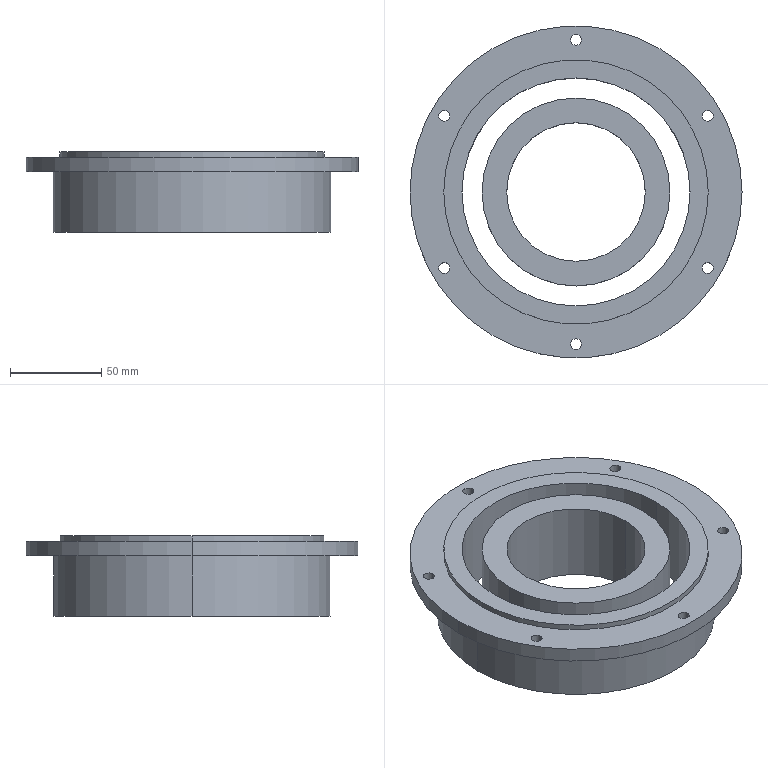Part | STEP file | Encoder | 2 solids | 30 faces | box 182 x 182 x 44 mm | volume 482174 mm3 | cylinder 24 | plane 6 | commonest cylinder face diameters 6 x12 76 x2 103 x2 125 x2 145 x2 152 x2
STEP:
#1=CARTESIAN_POINT('',(-51.5,0.,44.));
#2=VERTEX_POINT('',#1);
#3=CARTESIAN_POINT('',(51.5,0.,44.));
#4=VERTEX_POINT('',#3);
#5=CARTESIAN_POINT('',(0.,0.,44.));
#6=DIRECTION('',(0.,0.,-1.));
#7=DIRECTION('',(-1.,0.,0.));
#8=AXIS2_PLACEMENT_3D('',#5,#6,#7);
#9=CIRCLE('',#8,51.5);
#10=EDGE_CURVE('',#2,#4,#9,.T.);
#11=ORIENTED_EDGE('',*,*,#10,.T.);
#12=CARTESIAN_POINT('',(51.5,0.,0.));
#13=VERTEX_POINT('',#12);
#14=CARTESIAN_POINT('',(51.5,0.,44.));
#15=DIRECTION('',(0.,0.,-1.));
#16=VECTOR('',#15,1000.);
#17=LINE('',#14,#16);
#18=EDGE_CURVE('',#4,#13,#17,.T.);
#19=ORIENTED_EDGE('',*,*,#18,.T.);
#20=CARTESIAN_POINT('',(-51.5,0.,0.));
#21=VERTEX_POINT('',#20);
#22=CARTESIAN_POINT('',(0.,0.,0.));
#23=DIRECTION('',(0.,0.,1.));
#24=DIRECTION('',(-1.,0.,0.));
#25=AXIS2_PLACEMENT_3D('',#22,#23,#24);
#26=CIRCLE('',#25,51.5);
#27=EDGE_CURVE('',#13,#21,#26,.T.);
#28=ORIENTED_EDGE('',*,*,#27,.T.);
#29=CARTESIAN_POINT('',(-51.5,0.,44.));
#30=DIRECTION('',(0.,0.,-1.));
#31=VECTOR('',#30,1000.);
#32=LINE('',#29,#31);
#33=EDGE_CURVE('',#2,#21,#32,.T.);
#34=ORIENTED_EDGE('',*,*,#33,.F.);
#35=EDGE_LOOP('',(#11,#19,#28,#34));
#36=FACE_OUTER_BOUND('',#35,.T.);
#37=CARTESIAN_POINT('',(0.,0.,44.));
#38=DIRECTION('',(0.,0.,-1.));
#39=DIRECTION('',(-1.,0.,0.));
#40=AXIS2_PLACEMENT_3D('',#37,#38,#39);
#41=CYLINDRICAL_SURFACE('',#40,51.5);
#42=ADVANCED_FACE('',(#36),#41,.T.);
#43=CARTESIAN_POINT('',(38.,0.,44.));
#44=VERTEX_POINT('',#43);
#45=CARTESIAN_POINT('',(-38.,0.,44.));
#46=VERTEX_POINT('',#45);
#47=CARTESIAN_POINT('',(0.,0.,44.));
#48=DIRECTION('',(0.,0.,-1.));
#49=DIRECTION('',(-1.,0.,0.));
#50=AXIS2_PLACEMENT_3D('',#47,#48,#49);
#51=CIRCLE('',#50,38.);
#52=EDGE_CURVE('',#44,#46,#51,.T.);
#53=ORIENTED_EDGE('',*,*,#52,.F.);
#54=CARTESIAN_POINT('',(38.,0.,0.));
#55=VERTEX_POINT('',#54);
#56=CARTESIAN_POINT('',(38.,0.,41.));
#57=DIRECTION('',(0.,0.,-1.));
#58=VECTOR('',#57,1000.);
#59=LINE('',#56,#58);
#60=EDGE_CURVE('',#44,#55,#59,.T.);
#61=ORIENTED_EDGE('',*,*,#60,.T.);
#62=CARTESIAN_POINT('',(-38.,0.,0.));
#63=VERTEX_POINT('',#62);
#64=CARTESIAN_POINT('',(0.,0.,0.));
#65=DIRECTION('',(0.,0.,-1.));
#66=DIRECTION('',(-1.,0.,0.));
#67=AXIS2_PLACEMENT_3D('',#64,#65,#66);
#68=CIRCLE('',#67,38.);
#69=EDGE_CURVE('',#55,#63,#68,.T.);
#70=ORIENTED_EDGE('',*,*,#69,.T.);
#71=CARTESIAN_POINT('',(-38.,0.,41.));
#72=DIRECTION('',(0.,0.,-1.));
#73=VECTOR('',#72,1000.);
#74=LINE('',#71,#73);
#75=EDGE_CURVE('',#46,#63,#74,.T.);
#76=ORIENTED_EDGE('',*,*,#75,.F.);
#77=EDGE_LOOP('',(#53,#61,#70,#76));
#78=FACE_OUTER_BOUND('',#77,.T.);
#79=CARTESIAN_POINT('',(0.,0.,41.));
#80=DIRECTION('',(0.,0.,-1.));
#81=DIRECTION('',(-1.,0.,0.));
#82=AXIS2_PLACEMENT_3D('',#79,#80,#81);
#83=CYLINDRICAL_SURFACE('',#82,38.);
#84=ADVANCED_FACE('',(#78),#83,.F.);
#85=ORIENTED_EDGE('',*,*,#18,.F.);
#86=CARTESIAN_POINT('',(0.,0.,44.));
#87=DIRECTION('',(0.,0.,-1.));
#88=DIRECTION('',(-1.,0.,0.));
#89=AXIS2_PLACEMENT_3D('',#86,#87,#88);
#90=CIRCLE('',#89,51.5);
#91=EDGE_CURVE('',#4,#2,#90,.T.);
#92=ORIENTED_EDGE('',*,*,#91,.T.);
#93=ORIENTED_EDGE('',*,*,#33,.T.);
#94=CARTESIAN_POINT('',(0.,0.,0.));
#95=DIRECTION('',(0.,0.,1.));
#96=DIRECTION('',(-1.,0.,0.));
#97=AXIS2_PLACEMENT_3D('',#94,#95,#96);
#98=CIRCLE('',#97,51.5);
#99=EDGE_CURVE('',#21,#13,#98,.T.);
#100=ORIENTED_EDGE('',*,*,#99,.T.);
#101=EDGE_LOOP('',(#85,#92,#93,#100));
#102=FACE_OUTER_BOUND('',#101,.T.);
#103=CARTESIAN_POINT('',(0.,0.,44.));
#104=DIRECTION('',(0.,0.,-1.));
#105=DIRECTION('',(-1.,0.,0.));
#106=AXIS2_PLACEMENT_3D('',#103,#104,#105);
#107=CYLINDRICAL_SURFACE('',#106,51.5);
#108=ADVANCED_FACE('',(#102),#107,.T.);
#109=ORIENTED_EDGE('',*,*,#99,.F.);
#110=ORIENTED_EDGE('',*,*,#27,.F.);
#111=EDGE_LOOP('',(#109,#110));
#112=FACE_OUTER_BOUND('',#111,.T.);
#113=CARTESIAN_POINT('',(0.,0.,0.));
#114=DIRECTION('',(0.,0.,-1.));
#115=DIRECTION('',(-1.,0.,0.));
#116=AXIS2_PLACEMENT_3D('',#113,#114,#115);
#117=CIRCLE('',#116,38.);
#118=EDGE_CURVE('',#63,#55,#117,.T.);
#119=ORIENTED_EDGE('',*,*,#118,.F.);
#120=ORIENTED_EDGE('',*,*,#69,.F.);
#121=EDGE_LOOP('',(#119,#120));
#122=FACE_BOUND('',#121,.T.);
#123=CARTESIAN_POINT('',(0.,0.,0.));
#124=DIRECTION('',(0.,0.,1.));
#125=DIRECTION('',(1.,0.,0.));
#126=AXIS2_PLACEMENT_3D('',#123,#124,#125);
#127=PLANE('',#126);
#128=ADVANCED_FACE('',(#112,#122),#127,.F.);
#129=ORIENTED_EDGE('',*,*,#10,.F.);
#130=ORIENTED_EDGE('',*,*,#91,.F.);
#131=EDGE_LOOP('',(#129,#130));
#132=FACE_OUTER_BOUND('',#131,.T.);
#133=CARTESIAN_POINT('',(0.,0.,44.));
#134=DIRECTION('',(0.,0.,-1.));
#135=DIRECTION('',(-1.,0.,0.));
#136=AXIS2_PLACEMENT_3D('',#133,#134,#135);
#137=CIRCLE('',#136,38.);
#138=EDGE_CURVE('',#46,#44,#137,.T.);
#139=ORIENTED_EDGE('',*,*,#138,.T.);
#140=ORIENTED_EDGE('',*,*,#52,.T.);
#141=EDGE_LOOP('',(#139,#140));
#142=FACE_BOUND('',#141,.T.);
#143=CARTESIAN_POINT('',(0.,0.,44.));
#144=DIRECTION('',(0.,0.,1.));
#145=DIRECTION('',(1.,0.,0.));
#146=AXIS2_PLACEMENT_3D('',#143,#144,#145);
#147=PLANE('',#146);
#148=ADVANCED_FACE('',(#132,#142),#147,.T.);
#149=ORIENTED_EDGE('',*,*,#60,.F.);
#150=ORIENTED_EDGE('',*,*,#138,.F.);
#151=ORIENTED_EDGE('',*,*,#75,.T.);
#152=ORIENTED_EDGE('',*,*,#118,.T.);
#153=EDGE_LOOP('',(#149,#150,#151,#152));
#154=FACE_OUTER_BOUND('',#153,.T.);
#155=CARTESIAN_POINT('',(0.,0.,41.));
#156=DIRECTION('',(0.,0.,-1.));
#157=DIRECTION('',(-1.,0.,0.));
#158=AXIS2_PLACEMENT_3D('',#155,#156,#157);
#159=CYLINDRICAL_SURFACE('',#158,38.);
#160=ADVANCED_FACE('',(#154),#159,.F.);
#161=CLOSED_SHELL('',(#42,#84,#108,#128,#148,#160));
#162=MANIFOLD_SOLID_BREP('',#161);
#163=CARTESIAN_POINT('',(-72.5,0.,44.));
#164=VERTEX_POINT('',#163);
#165=CARTESIAN_POINT('',(72.5,0.,44.));
#166=VERTEX_POINT('',#165);
#167=CARTESIAN_POINT('',(0.,0.,44.));
#168=DIRECTION('',(0.,0.,-1.));
#169=DIRECTION('',(-1.,0.,0.));
#170=AXIS2_PLACEMENT_3D('',#167,#168,#169);
#171=CIRCLE('',#170,72.5);
#172=EDGE_CURVE('',#164,#166,#171,.T.);
#173=ORIENTED_EDGE('',*,*,#172,.T.);
#174=CARTESIAN_POINT('',(72.5,0.,41.));
#175=VERTEX_POINT('',#174);
#176=CARTESIAN_POINT('',(72.5,0.,44.));
#177=DIRECTION('',(0.,0.,-1.));
#178=VECTOR('',#177,1000.);
#179=LINE('',#176,#178);
#180=EDGE_CURVE('',#166,#175,#179,.T.);
#181=ORIENTED_EDGE('',*,*,#180,.T.);
#182=CARTESIAN_POINT('',(-72.5,0.,41.));
#183=VERTEX_POINT('',#182);
#184=CARTESIAN_POINT('',(0.,0.,41.));
#185=DIRECTION('',(0.,0.,-1.));
#186=DIRECTION('',(-1.,0.,0.));
#187=AXIS2_PLACEMENT_3D('',#184,#185,#186);
#188=CIRCLE('',#187,72.5);
#189=EDGE_CURVE('',#183,#175,#188,.T.);
#190=ORIENTED_EDGE('',*,*,#189,.F.);
#191=CARTESIAN_POINT('',(-72.5,0.,44.));
#192=DIRECTION('',(0.,0.,-1.));
#193=VECTOR('',#192,1000.);
#194=LINE('',#191,#193);
#195=EDGE_CURVE('',#164,#183,#194,.T.);
#196=ORIENTED_EDGE('',*,*,#195,.F.);
#197=EDGE_LOOP('',(#173,#181,#190,#196));
#198=FACE_OUTER_BOUND('',#197,.T.);
#199=CARTESIAN_POINT('',(0.,0.,44.));
#200=DIRECTION('',(0.,0.,-1.));
#201=DIRECTION('',(-1.,0.,0.));
#202=AXIS2_PLACEMENT_3D('',#199,#200,#201);
#203=CYLINDRICAL_SURFACE('',#202,72.5);
#204=ADVANCED_FACE('',(#198),#203,.T.);
#205=CARTESIAN_POINT('',(91.,0.,41.));
#206=VERTEX_POINT('',#205);
#207=CARTESIAN_POINT('',(-91.,0.,41.));
#208=VERTEX_POINT('',#207);
#209=CARTESIAN_POINT('',(0.,0.,41.));
#210=DIRECTION('',(0.,0.,1.));
#211=DIRECTION('',(-1.,0.,0.));
#212=AXIS2_PLACEMENT_3D('',#209,#210,#211);
#213=CIRCLE('',#212,91.);
#214=EDGE_CURVE('',#206,#208,#213,.T.);
#215=ORIENTED_EDGE('',*,*,#214,.F.);
#216=CARTESIAN_POINT('',(91.,0.,33.));
#217=VERTEX_POINT('',#216);
#218=CARTESIAN_POINT('',(91.,0.,41.));
#219=DIRECTION('',(0.,0.,-1.));
#220=VECTOR('',#219,1000.);
#221=LINE('',#218,#220);
#222=EDGE_CURVE('',#206,#217,#221,.T.);
#223=ORIENTED_EDGE('',*,*,#222,.T.);
#224=CARTESIAN_POINT('',(-91.,0.,33.));
#225=VERTEX_POINT('',#224);
#226=CARTESIAN_POINT('',(0.,0.,33.));
#227=DIRECTION('',(0.,0.,1.));
#228=DIRECTION('',(-1.,0.,0.));
#229=AXIS2_PLACEMENT_3D('',#226,#227,#228);
#230=CIRCLE('',#229,91.);
#231=EDGE_CURVE('',#217,#225,#230,.T.);
#232=ORIENTED_EDGE('',*,*,#231,.T.);
#233=CARTESIAN_POINT('',(-91.,0.,41.));
#234=DIRECTION('',(0.,0.,-1.));
#235=VECTOR('',#234,1000.);
#236=LINE('',#233,#235);
#237=EDGE_CURVE('',#208,#225,#236,.T.);
#238=ORIENTED_EDGE('',*,*,#237,.F.);
#239=EDGE_LOOP('',(#215,#223,#232,#238));
#240=FACE_OUTER_BOUND('',#239,.T.);
#241=CARTESIAN_POINT('',(0.,0.,41.));
#242=DIRECTION('',(0.,0.,-1.));
#243=DIRECTION('',(-1.,0.,0.));
#244=AXIS2_PLACEMENT_3D('',#241,#242,#243);
#245=CYLINDRICAL_SURFACE('',#244,91.);
#246=ADVANCED_FACE('',(#240),#245,.T.);
#247=CARTESIAN_POINT('',(3.,83.44,41.));
#248=VERTEX_POINT('',#247);
#249=CARTESIAN_POINT('',(-3.,83.44,41.));
#250=VERTEX_POINT('',#249);
#251=CARTESIAN_POINT('',(0.,83.44,41.));
#252=DIRECTION('',(0.,0.,-1.));
#253=DIRECTION('',(-1.,0.,0.));
#254=AXIS2_PLACEMENT_3D('',#251,#252,#253);
#255=CIRCLE('',#254,3.);
#256=EDGE_CURVE('',#248,#250,#255,.T.);
#257=ORIENTED_EDGE('',*,*,#256,.F.);
#258=CARTESIAN_POINT('',(3.,83.44,33.));
#259=VERTEX_POINT('',#258);
#260=CARTESIAN_POINT('',(3.,83.44,44.));
#261=DIRECTION('',(0.,0.,-1.));
#262=VECTOR('',#261,1000.);
#263=LINE('',#260,#262);
#264=EDGE_CURVE('',#248,#259,#263,.T.);
#265=ORIENTED_EDGE('',*,*,#264,.T.);
#266=CARTESIAN_POINT('',(-3.,83.44,33.));
#267=VERTEX_POINT('',#266);
#268=CARTESIAN_POINT('',(0.,83.44,33.));
#269=DIRECTION('',(0.,0.,1.));
#270=DIRECTION('',(-1.,0.,0.));
#271=AXIS2_PLACEMENT_3D('',#268,#269,#270);
#272=CIRCLE('',#271,3.);
#273=EDGE_CURVE('',#267,#259,#272,.T.);
#274=ORIENTED_EDGE('',*,*,#273,.F.);
#275=CARTESIAN_POINT('',(-3.,83.44,44.));
#276=DIRECTION('',(0.,0.,-1.));
#277=VECTOR('',#276,1000.);
#278=LINE('',#275,#277);
#279=EDGE_CURVE('',#250,#267,#278,.T.);
#280=ORIENTED_EDGE('',*,*,#279,.F.);
#281=EDGE_LOOP('',(#257,#265,#274,#280));
#282=FACE_OUTER_BOUND('',#281,.T.);
#283=CARTESIAN_POINT('',(0.,83.44,44.));
#284=DIRECTION('',(0.,0.,-1.));
#285=DIRECTION('',(-1.,0.,0.));
#286=AXIS2_PLACEMENT_3D('',#283,#284,#285);
#287=CYLINDRICAL_SURFACE('',#286,3.);
#288=ADVANCED_FACE('',(#282),#287,.F.);
#289=CARTESIAN_POINT('',(-69.261,41.72,41.));
#290=VERTEX_POINT('',#289);
#291=CARTESIAN_POINT('',(-75.261,41.72,41.));
#292=VERTEX_POINT('',#291);
#293=CARTESIAN_POINT('',(-72.261,41.72,41.));
#294=DIRECTION('',(0.,0.,-1.));
#295=DIRECTION('',(-1.,0.,0.));
#296=AXIS2_PLACEMENT_3D('',#293,#294,#295);
#297=CIRCLE('',#296,3.);
#298=EDGE_CURVE('',#290,#292,#297,.T.);
#299=ORIENTED_EDGE('',*,*,#298,.F.);
#300=CARTESIAN_POINT('',(-69.261,41.72,33.));
#301=VERTEX_POINT('',#300);
#302=CARTESIAN_POINT('',(-69.261,41.72,44.));
#303=DIRECTION('',(0.,0.,-1.));
#304=VECTOR('',#303,1000.);
#305=LINE('',#302,#304);
#306=EDGE_CURVE('',#290,#301,#305,.T.);
#307=ORIENTED_EDGE('',*,*,#306,.T.);
#308=CARTESIAN_POINT('',(-75.261,41.72,33.));
#309=VERTEX_POINT('',#308);
#310=CARTESIAN_POINT('',(-72.261,41.72,33.));
#311=DIRECTION('',(0.,0.,1.));
#312=DIRECTION('',(-1.,0.,0.));
#313=AXIS2_PLACEMENT_3D('',#310,#311,#312);
#314=CIRCLE('',#313,3.);
#315=EDGE_CURVE('',#309,#301,#314,.T.);
#316=ORIENTED_EDGE('',*,*,#315,.F.);
#317=CARTESIAN_POINT('',(-75.261,41.72,44.));
#318=DIRECTION('',(0.,0.,-1.));
#319=VECTOR('',#318,1000.);
#320=LINE('',#317,#319);
#321=EDGE_CURVE('',#292,#309,#320,.T.);
#322=ORIENTED_EDGE('',*,*,#321,.F.);
#323=EDGE_LOOP('',(#299,#307,#316,#322));
#324=FACE_OUTER_BOUND('',#323,.T.);
#325=CARTESIAN_POINT('',(-72.261,41.72,44.));
#326=DIRECTION('',(0.,0.,-1.));
#327=DIRECTION('',(-1.,0.,0.));
#328=AXIS2_PLACEMENT_3D('',#325,#326,#327);
#329=CYLINDRICAL_SURFACE('',#328,3.);
#330=ADVANCED_FACE('',(#324),#329,.F.);
#331=CARTESIAN_POINT('',(-69.261,-41.72,41.));
#332=VERTEX_POINT('',#331);
#333=CARTESIAN_POINT('',(-75.261,-41.72,41.));
#334=VERTEX_POINT('',#333);
#335=CARTESIAN_POINT('',(-72.261,-41.72,41.));
#336=DIRECTION('',(0.,0.,-1.));
#337=DIRECTION('',(-1.,0.,0.));
#338=AXIS2_PLACEMENT_3D('',#335,#336,#337);
#339=CIRCLE('',#338,3.);
#340=EDGE_CURVE('',#332,#334,#339,.T.);
#341=ORIENTED_EDGE('',*,*,#340,.F.);
#342=CARTESIAN_POINT('',(-69.261,-41.72,33.));
#343=VERTEX_POINT('',#342);
#344=CARTESIAN_POINT('',(-69.261,-41.72,44.));
#345=DIRECTION('',(0.,0.,-1.));
#346=VECTOR('',#345,1000.);
#347=LINE('',#344,#346);
#348=EDGE_CURVE('',#332,#343,#347,.T.);
#349=ORIENTED_EDGE('',*,*,#348,.T.);
#350=CARTESIAN_POINT('',(-75.261,-41.72,33.));
#351=VERTEX_POINT('',#350);
#352=CARTESIAN_POINT('',(-72.261,-41.72,33.));
#353=DIRECTION('',(0.,0.,1.));
#354=DIRECTION('',(-1.,0.,0.));
#355=AXIS2_PLACEMENT_3D('',#352,#353,#354);
#356=CIRCLE('',#355,3.);
#357=EDGE_CURVE('',#351,#343,#356,.T.);
#358=ORIENTED_EDGE('',*,*,#357,.F.);
#359=CARTESIAN_POINT('',(-75.261,-41.72,44.));
#360=DIRECTION('',(0.,0.,-1.));
#361=VECTOR('',#360,1000.);
#362=LINE('',#359,#361);
#363=EDGE_CURVE('',#334,#351,#362,.T.);
#364=ORIENTED_EDGE('',*,*,#363,.F.);
#365=EDGE_LOOP('',(#341,#349,#358,#364));
#366=FACE_OUTER_BOUND('',#365,.T.);
#367=CARTESIAN_POINT('',(-72.261,-41.72,44.));
#368=DIRECTION('',(0.,0.,-1.));
#369=DIRECTION('',(-1.,0.,0.));
#370=AXIS2_PLACEMENT_3D('',#367,#368,#369);
#371=CYLINDRICAL_SURFACE('',#370,3.);
#372=ADVANCED_FACE('',(#366),#371,.F.);
#373=CARTESIAN_POINT('',(3.,-83.44,41.));
#374=VERTEX_POINT('',#373);
#375=CARTESIAN_POINT('',(-3.,-83.44,41.));
#376=VERTEX_POINT('',#375);
#377=CARTESIAN_POINT('',(0.,-83.44,41.));
#378=DIRECTION('',(0.,0.,-1.));
#379=DIRECTION('',(-1.,0.,0.));
#380=AXIS2_PLACEMENT_3D('',#377,#378,#379);
#381=CIRCLE('',#380,3.);
#382=EDGE_CURVE('',#374,#376,#381,.T.);
#383=ORIENTED_EDGE('',*,*,#382,.F.);
#384=CARTESIAN_POINT('',(3.,-83.44,33.));
#385=VERTEX_POINT('',#384);
#386=CARTESIAN_POINT('',(3.,-83.44,44.));
#387=DIRECTION('',(0.,0.,-1.));
#388=VECTOR('',#387,1000.);
#389=LINE('',#386,#388);
#390=EDGE_CURVE('',#374,#385,#389,.T.);
#391=ORIENTED_EDGE('',*,*,#390,.T.);
#392=CARTESIAN_POINT('',(-3.,-83.44,33.));
#393=VERTEX_POINT('',#392);
#394=CARTESIAN_POINT('',(0.,-83.44,33.));
#395=DIRECTION('',(0.,0.,1.));
#396=DIRECTION('',(-1.,0.,0.));
#397=AXIS2_PLACEMENT_3D('',#394,#395,#396);
#398=CIRCLE('',#397,3.);
#399=EDGE_CURVE('',#393,#385,#398,.T.);
#400=ORIENTED_EDGE('',*,*,#399,.F.);
#401=CARTESIAN_POINT('',(-3.,-83.44,44.));
#402=DIRECTION('',(0.,0.,-1.));
#403=VECTOR('',#402,1000.);
#404=LINE('',#401,#403);
#405=EDGE_CURVE('',#376,#393,#404,.T.);
#406=ORIENTED_EDGE('',*,*,#405,.F.);
#407=EDGE_LOOP('',(#383,#391,#400,#406));
#408=FACE_OUTER_BOUND('',#407,.T.);
#409=CARTESIAN_POINT('',(0.,-83.44,44.));
#410=DIRECTION('',(0.,0.,-1.));
#411=DIRECTION('',(-1.,0.,0.));
#412=AXIS2_PLACEMENT_3D('',#409,#410,#411);
#413=CYLINDRICAL_SURFACE('',#412,3.);
#414=ADVANCED_FACE('',(#408),#413,.F.);
#415=CARTESIAN_POINT('',(75.261,-41.72,41.));
#416=VERTEX_POINT('',#415);
#417=CARTESIAN_POINT('',(69.261,-41.72,41.));
#418=VERTEX_POINT('',#417);
#419=CARTESIAN_POINT('',(72.261,-41.72,41.));
#420=DIRECTION('',(0.,0.,-1.));
#421=DIRECTION('',(-1.,0.,0.));
#422=AXIS2_PLACEMENT_3D('',#419,#420,#421);
#423=CIRCLE('',#422,3.);
#424=EDGE_CURVE('',#416,#418,#423,.T.);
#425=ORIENTED_EDGE('',*,*,#424,.F.);
#426=CARTESIAN_POINT('',(75.261,-41.72,33.));
#427=VERTEX_POINT('',#426);
#428=CARTESIAN_POINT('',(75.261,-41.72,44.));
#429=DIRECTION('',(0.,0.,-1.));
#430=VECTOR('',#429,1000.);
#431=LINE('',#428,#430);
#432=EDGE_CURVE('',#416,#427,#431,.T.);
#433=ORIENTED_EDGE('',*,*,#432,.T.);
#434=CARTESIAN_POINT('',(69.261,-41.72,33.));
#435=VERTEX_POINT('',#434);
#436=CARTESIAN_POINT('',(72.261,-41.72,33.));
#437=DIRECTION('',(0.,0.,1.));
#438=DIRECTION('',(-1.,0.,0.));
#439=AXIS2_PLACEMENT_3D('',#436,#437,#438);
#440=CIRCLE('',#439,3.);
#441=EDGE_CURVE('',#435,#427,#440,.T.);
#442=ORIENTED_EDGE('',*,*,#441,.F.);
#443=CARTESIAN_POINT('',(69.261,-41.72,44.));
#444=DIRECTION('',(0.,0.,-1.));
#445=VECTOR('',#444,1000.);
#446=LINE('',#443,#445);
#447=EDGE_CURVE('',#418,#435,#446,.T.);
#448=ORIENTED_EDGE('',*,*,#447,.F.);
#449=EDGE_LOOP('',(#425,#433,#442,#448));
#450=FACE_OUTER_BOUND('',#449,.T.);
#451=CARTESIAN_POINT('',(72.261,-41.72,44.));
#452=DIRECTION('',(0.,0.,-1.));
#453=DIRECTION('',(-1.,0.,0.));
#454=AXIS2_PLACEMENT_3D('',#451,#452,#453);
#455=CYLINDRICAL_SURFACE('',#454,3.);
#456=ADVANCED_FACE('',(#450),#455,.F.);
#457=CARTESIAN_POINT('',(75.261,41.72,41.));
#458=VERTEX_POINT('',#457);
#459=CARTESIAN_POINT('',(69.261,41.72,41.));
#460=VERTEX_POINT('',#459);
#461=CARTESIAN_POINT('',(72.261,41.72,41.));
#462=DIRECTION('',(0.,0.,-1.));
#463=DIRECTION('',(-1.,0.,0.));
#464=AXIS2_PLACEMENT_3D('',#461,#462,#463);
#465=CIRCLE('',#464,3.);
#466=EDGE_CURVE('',#458,#460,#465,.T.);
#467=ORIENTED_EDGE('',*,*,#466,.F.);
#468=CARTESIAN_POINT('',(75.261,41.72,33.));
#469=VERTEX_POINT('',#468);
#470=CARTESIAN_POINT('',(75.261,41.72,44.));
#471=DIRECTION('',(0.,0.,-1.));
#472=VECTOR('',#471,1000.);
#473=LINE('',#470,#472);
#474=EDGE_CURVE('',#458,#469,#473,.T.);
#475=ORIENTED_EDGE('',*,*,#474,.T.);
#476=CARTESIAN_POINT('',(69.261,41.72,33.));
#477=VERTEX_POINT('',#476);
#478=CARTESIAN_POINT('',(72.261,41.72,33.));
#479=DIRECTION('',(0.,0.,1.));
#480=DIRECTION('',(-1.,0.,0.));
#481=AXIS2_PLACEMENT_3D('',#478,#479,#480);
#482=CIRCLE('',#481,3.);
#483=EDGE_CURVE('',#477,#469,#482,.T.);
#484=ORIENTED_EDGE('',*,*,#483,.F.);
#485=CARTESIAN_POINT('',(69.261,41.72,44.));
#486=DIRECTION('',(0.,0.,-1.));
#487=VECTOR('',#486,1000.);
#488=LINE('',#485,#487);
#489=EDGE_CURVE('',#460,#477,#488,.T.);
#490=ORIENTED_EDGE('',*,*,#489,.F.);
#491=EDGE_LOOP('',(#467,#475,#484,#490));
#492=FACE_OUTER_BOUND('',#491,.T.);
#493=CARTESIAN_POINT('',(72.261,41.72,44.));
#494=DIRECTION('',(0.,0.,-1.));
#495=DIRECTION('',(-1.,0.,0.));
#496=AXIS2_PLACEMENT_3D('',#493,#494,#495);
#497=CYLINDRICAL_SURFACE('',#496,3.);
#498=ADVANCED_FACE('',(#492),#497,.F.);
#499=CARTESIAN_POINT('',(62.5,0.,44.));
#500=VERTEX_POINT('',#499);
#501=CARTESIAN_POINT('',(-62.5,0.,44.));
#502=VERTEX_POINT('',#501);
#503=CARTESIAN_POINT('',(0.,0.,44.));
#504=DIRECTION('',(0.,0.,-1.));
#505=DIRECTION('',(-1.,0.,0.));
#506=AXIS2_PLACEMENT_3D('',#503,#504,#505);
#507=CIRCLE('',#506,62.5);
#508=EDGE_CURVE('',#500,#502,#507,.T.);
#509=ORIENTED_EDGE('',*,*,#508,.F.);
#510=CARTESIAN_POINT('',(62.5,0.,0.));
#511=VERTEX_POINT('',#510);
#512=CARTESIAN_POINT('',(62.5,0.,44.));
#513=DIRECTION('',(0.,0.,-1.));
#514=VECTOR('',#513,1000.);
#515=LINE('',#512,#514);
#516=EDGE_CURVE('',#500,#511,#515,.T.);
#517=ORIENTED_EDGE('',*,*,#516,.T.);
#518=CARTESIAN_POINT('',(-62.5,0.,0.));
#519=VERTEX_POINT('',#518);
#520=CARTESIAN_POINT('',(0.,0.,0.));
#521=DIRECTION('',(0.,0.,1.));
#522=DIRECTION('',(-1.,0.,0.));
#523=AXIS2_PLACEMENT_3D('',#520,#521,#522);
#524=CIRCLE('',#523,62.5);
#525=EDGE_CURVE('',#519,#511,#524,.T.);
#526=ORIENTED_EDGE('',*,*,#525,.F.);
#527=CARTESIAN_POINT('',(-62.5,0.,44.));
#528=DIRECTION('',(0.,0.,-1.));
#529=VECTOR('',#528,1000.);
#530=LINE('',#527,#529);
#531=EDGE_CURVE('',#502,#519,#530,.T.);
#532=ORIENTED_EDGE('',*,*,#531,.F.);
#533=EDGE_LOOP('',(#509,#517,#526,#532));
#534=FACE_OUTER_BOUND('',#533,.T.);
#535=CARTESIAN_POINT('',(0.,0.,44.));
#536=DIRECTION('',(0.,0.,-1.));
#537=DIRECTION('',(-1.,0.,0.));
#538=AXIS2_PLACEMENT_3D('',#535,#536,#537);
#539=CYLINDRICAL_SURFACE('',#538,62.5);
#540=ADVANCED_FACE('',(#534),#539,.F.);
#541=CARTESIAN_POINT('',(76.,0.,33.));
#542=VERTEX_POINT('',#541);
#543=CARTESIAN_POINT('',(-76.,0.,33.));
#544=VERTEX_POINT('',#543);
#545=CARTESIAN_POINT('',(0.,0.,33.));
#546=DIRECTION('',(0.,0.,1.));
#547=DIRECTION('',(-1.,0.,0.));
#548=AXIS2_PLACEMENT_3D('',#545,#546,#547);
#549=CIRCLE('',#548,76.);
#550=EDGE_CURVE('',#542,#544,#549,.T.);
#551=ORIENTED_EDGE('',*,*,#550,.F.);
#552=CARTESIAN_POINT('',(76.,0.,0.));
#553=VERTEX_POINT('',#552);
#554=CARTESIAN_POINT('',(76.,0.,33.));
#555=DIRECTION('',(0.,0.,-1.));
#556=VECTOR('',#555,1000.);
#557=LINE('',#554,#556);
#558=EDGE_CURVE('',#542,#553,#557,.T.);
#559=ORIENTED_EDGE('',*,*,#558,.T.);
#560=CARTESIAN_POINT('',(-76.,0.,0.));
#561=VERTEX_POINT('',#560);
#562=CARTESIAN_POINT('',(0.,0.,0.));
#563=DIRECTION('',(0.,0.,1.));
#564=DIRECTION('',(-1.,0.,0.));
#565=AXIS2_PLACEMENT_3D('',#562,#563,#564);
#566=CIRCLE('',#565,76.);
#567=EDGE_CURVE('',#553,#561,#566,.T.);
#568=ORIENTED_EDGE('',*,*,#567,.T.);
#569=CARTESIAN_POINT('',(-76.,0.,33.));
#570=DIRECTION('',(0.,0.,-1.));
#571=VECTOR('',#570,1000.);
#572=LINE('',#569,#571);
#573=EDGE_CURVE('',#544,#561,#572,.T.);
#574=ORIENTED_EDGE('',*,*,#573,.F.);
#575=EDGE_LOOP('',(#551,#559,#568,#574));
#576=FACE_OUTER_BOUND('',#575,.T.);
#577=CARTESIAN_POINT('',(0.,0.,33.));
#578=DIRECTION('',(0.,0.,-1.));
#579=DIRECTION('',(-1.,0.,0.));
#580=AXIS2_PLACEMENT_3D('',#577,#578,#579);
#581=CYLINDRICAL_SURFACE('',#580,76.);
#582=ADVANCED_FACE('',(#576),#581,.T.);
#583=ORIENTED_EDGE('',*,*,#189,.T.);
#584=CARTESIAN_POINT('',(0.,0.,41.));
#585=DIRECTION('',(0.,0.,-1.));
#586=DIRECTION('',(-1.,0.,0.));
#587=AXIS2_PLACEMENT_3D('',#584,#585,#586);
#588=CIRCLE('',#587,72.5);
#589=EDGE_CURVE('',#175,#183,#588,.T.);
#590=ORIENTED_EDGE('',*,*,#589,.T.);
#591=EDGE_LOOP('',(#583,#590));
#592=FACE_BOUND('',#591,.T.);
#593=CARTESIAN_POINT('',(0.,0.,41.));
#594=DIRECTION('',(0.,0.,1.));
#595=DIRECTION('',(-1.,0.,0.));
#596=AXIS2_PLACEMENT_3D('',#593,#594,#595);
#597=CIRCLE('',#596,91.);
#598=EDGE_CURVE('',#208,#206,#597,.T.);
#599=ORIENTED_EDGE('',*,*,#598,.T.);
#600=ORIENTED_EDGE('',*,*,#214,.T.);
#601=EDGE_LOOP('',(#599,#600));
#602=FACE_OUTER_BOUND('',#601,.T.);
#603=CARTESIAN_POINT('',(0.,83.44,41.));
#604=DIRECTION('',(0.,0.,-1.));
#605=DIRECTION('',(-1.,0.,0.));
#606=AXIS2_PLACEMENT_3D('',#603,#604,#605);
#607=CIRCLE('',#606,3.);
#608=EDGE_CURVE('',#250,#248,#607,.T.);
#609=ORIENTED_EDGE('',*,*,#608,.T.);
#610=ORIENTED_EDGE('',*,*,#256,.T.);
#611=EDGE_LOOP('',(#609,#610));
#612=FACE_BOUND('',#611,.T.);
#613=CARTESIAN_POINT('',(-72.261,41.72,41.));
#614=DIRECTION('',(0.,0.,-1.));
#615=DIRECTION('',(-1.,0.,0.));
#616=AXIS2_PLACEMENT_3D('',#613,#614,#615);
#617=CIRCLE('',#616,3.);
#618=EDGE_CURVE('',#292,#290,#617,.T.);
#619=ORIENTED_EDGE('',*,*,#618,.T.);
#620=ORIENTED_EDGE('',*,*,#298,.T.);
#621=EDGE_LOOP('',(#619,#620));
#622=FACE_BOUND('',#621,.T.);
#623=CARTESIAN_POINT('',(-72.261,-41.72,41.));
#624=DIRECTION('',(0.,0.,-1.));
#625=DIRECTION('',(-1.,0.,0.));
#626=AXIS2_PLACEMENT_3D('',#623,#624,#625);
#627=CIRCLE('',#626,3.);
#628=EDGE_CURVE('',#334,#332,#627,.T.);
#629=ORIENTED_EDGE('',*,*,#628,.T.);
#630=ORIENTED_EDGE('',*,*,#340,.T.);
#631=EDGE_LOOP('',(#629,#630));
#632=FACE_BOUND('',#631,.T.);
#633=CARTESIAN_POINT('',(0.,-83.44,41.));
#634=DIRECTION('',(0.,0.,-1.));
#635=DIRECTION('',(-1.,0.,0.));
#636=AXIS2_PLACEMENT_3D('',#633,#634,#635);
#637=CIRCLE('',#636,3.);
#638=EDGE_CURVE('',#376,#374,#637,.T.);
#639=ORIENTED_EDGE('',*,*,#638,.T.);
#640=ORIENTED_EDGE('',*,*,#382,.T.);
#641=EDGE_LOOP('',(#639,#640));
#642=FACE_BOUND('',#641,.T.);
#643=CARTESIAN_POINT('',(72.261,-41.72,41.));
#644=DIRECTION('',(0.,0.,-1.));
#645=DIRECTION('',(-1.,0.,0.));
#646=AXIS2_PLACEMENT_3D('',#643,#644,#645);
#647=CIRCLE('',#646,3.);
#648=EDGE_CURVE('',#418,#416,#647,.T.);
#649=ORIENTED_EDGE('',*,*,#648,.T.);
#650=ORIENTED_EDGE('',*,*,#424,.T.);
#651=EDGE_LOOP('',(#649,#650));
#652=FACE_BOUND('',#651,.T.);
#653=CARTESIAN_POINT('',(72.261,41.72,41.));
#654=DIRECTION('',(0.,0.,-1.));
#655=DIRECTION('',(-1.,0.,0.));
#656=AXIS2_PLACEMENT_3D('',#653,#654,#655);
#657=CIRCLE('',#656,3.);
#658=EDGE_CURVE('',#460,#458,#657,.T.);
#659=ORIENTED_EDGE('',*,*,#658,.T.);
#660=ORIENTED_EDGE('',*,*,#466,.T.);
#661=EDGE_LOOP('',(#659,#660));
#662=FACE_BOUND('',#661,.T.);
#663=CARTESIAN_POINT('',(0.,0.,41.));
#664=DIRECTION('',(0.,0.,1.));
#665=DIRECTION('',(1.,0.,0.));
#666=AXIS2_PLACEMENT_3D('',#663,#664,#665);
#667=PLANE('',#666);
#668=ADVANCED_FACE('',(#592,#602,#612,#622,#632,#642,#652,#662),#667,.T.);
#669=ORIENTED_EDGE('',*,*,#180,.F.);
#670=CARTESIAN_POINT('',(0.,0.,44.));
#671=DIRECTION('',(0.,0.,-1.));
#672=DIRECTION('',(-1.,0.,0.));
#673=AXIS2_PLACEMENT_3D('',#670,#671,#672);
#674=CIRCLE('',#673,72.5);
#675=EDGE_CURVE('',#166,#164,#674,.T.);
#676=ORIENTED_EDGE('',*,*,#675,.T.);
#677=ORIENTED_EDGE('',*,*,#195,.T.);
#678=ORIENTED_EDGE('',*,*,#589,.F.);
#679=EDGE_LOOP('',(#669,#676,#677,#678));
#680=FACE_OUTER_BOUND('',#679,.T.);
#681=CARTESIAN_POINT('',(0.,0.,44.));
#682=DIRECTION('',(0.,0.,-1.));
#683=DIRECTION('',(-1.,0.,0.));
#684=AXIS2_PLACEMENT_3D('',#681,#682,#683);
#685=CYLINDRICAL_SURFACE('',#684,72.5);
#686=ADVANCED_FACE('',(#680),#685,.T.);
#687=ORIENTED_EDGE('',*,*,#222,.F.);
#688=ORIENTED_EDGE('',*,*,#598,.F.);
#689=ORIENTED_EDGE('',*,*,#237,.T.);
#690=CARTESIAN_POINT('',(0.,0.,33.));
#691=DIRECTION('',(0.,0.,1.));
#692=DIRECTION('',(-1.,0.,0.));
#693=AXIS2_PLACEMENT_3D('',#690,#691,#692);
#694=CIRCLE('',#693,91.);
#695=EDGE_CURVE('',#225,#217,#694,.T.);
#696=ORIENTED_EDGE('',*,*,#695,.T.);
#697=EDGE_LOOP('',(#687,#688,#689,#696));
#698=FACE_OUTER_BOUND('',#697,.T.);
#699=CARTESIAN_POINT('',(0.,0.,41.));
#700=DIRECTION('',(0.,0.,-1.));
#701=DIRECTION('',(-1.,0.,0.));
#702=AXIS2_PLACEMENT_3D('',#699,#700,#701);
#703=CYLINDRICAL_SURFACE('',#702,91.);
#704=ADVANCED_FACE('',(#698),#703,.T.);
#705=ORIENTED_EDGE('',*,*,#264,.F.);
#706=ORIENTED_EDGE('',*,*,#608,.F.);
#707=ORIENTED_EDGE('',*,*,#279,.T.);
#708=CARTESIAN_POINT('',(0.,83.44,33.));
#709=DIRECTION('',(0.,0.,1.));
#710=DIRECTION('',(-1.,0.,0.));
#711=AXIS2_PLACEMENT_3D('',#708,#709,#710);
#712=CIRCLE('',#711,3.);
#713=EDGE_CURVE('',#259,#267,#712,.T.);
#714=ORIENTED_EDGE('',*,*,#713,.F.);
#715=EDGE_LOOP('',(#705,#706,#707,#714));
#716=FACE_OUTER_BOUND('',#715,.T.);
#717=CARTESIAN_POINT('',(0.,83.44,44.));
#718=DIRECTION('',(0.,0.,-1.));
#719=DIRECTION('',(-1.,0.,0.));
#720=AXIS2_PLACEMENT_3D('',#717,#718,#719);
#721=CYLINDRICAL_SURFACE('',#720,3.);
#722=ADVANCED_FACE('',(#716),#721,.F.);
#723=ORIENTED_EDGE('',*,*,#306,.F.);
#724=ORIENTED_EDGE('',*,*,#618,.F.);
#725=ORIENTED_EDGE('',*,*,#321,.T.);
#726=CARTESIAN_POINT('',(-72.261,41.72,33.));
#727=DIRECTION('',(0.,0.,1.));
#728=DIRECTION('',(-1.,0.,0.));
#729=AXIS2_PLACEMENT_3D('',#726,#727,#728);
#730=CIRCLE('',#729,3.);
#731=EDGE_CURVE('',#301,#309,#730,.T.);
#732=ORIENTED_EDGE('',*,*,#731,.F.);
#733=EDGE_LOOP('',(#723,#724,#725,#732));
#734=FACE_OUTER_BOUND('',#733,.T.);
#735=CARTESIAN_POINT('',(-72.261,41.72,44.));
#736=DIRECTION('',(0.,0.,-1.));
#737=DIRECTION('',(-1.,0.,0.));
#738=AXIS2_PLACEMENT_3D('',#735,#736,#737);
#739=CYLINDRICAL_SURFACE('',#738,3.);
#740=ADVANCED_FACE('',(#734),#739,.F.);
#741=ORIENTED_EDGE('',*,*,#348,.F.);
#742=ORIENTED_EDGE('',*,*,#628,.F.);
#743=ORIENTED_EDGE('',*,*,#363,.T.);
#744=CARTESIAN_POINT('',(-72.261,-41.72,33.));
#745=DIRECTION('',(0.,0.,1.));
#746=DIRECTION('',(-1.,0.,0.));
#747=AXIS2_PLACEMENT_3D('',#744,#745,#746);
#748=CIRCLE('',#747,3.);
#749=EDGE_CURVE('',#343,#351,#748,.T.);
#750=ORIENTED_EDGE('',*,*,#749,.F.);
#751=EDGE_LOOP('',(#741,#742,#743,#750));
#752=FACE_OUTER_BOUND('',#751,.T.);
#753=CARTESIAN_POINT('',(-72.261,-41.72,44.));
#754=DIRECTION('',(0.,0.,-1.));
#755=DIRECTION('',(-1.,0.,0.));
#756=AXIS2_PLACEMENT_3D('',#753,#754,#755);
#757=CYLINDRICAL_SURFACE('',#756,3.);
#758=ADVANCED_FACE('',(#752),#757,.F.);
#759=ORIENTED_EDGE('',*,*,#390,.F.);
#760=ORIENTED_EDGE('',*,*,#638,.F.);
#761=ORIENTED_EDGE('',*,*,#405,.T.);
#762=CARTESIAN_POINT('',(0.,-83.44,33.));
#763=DIRECTION('',(0.,0.,1.));
#764=DIRECTION('',(-1.,0.,0.));
#765=AXIS2_PLACEMENT_3D('',#762,#763,#764);
#766=CIRCLE('',#765,3.);
#767=EDGE_CURVE('',#385,#393,#766,.T.);
#768=ORIENTED_EDGE('',*,*,#767,.F.);
#769=EDGE_LOOP('',(#759,#760,#761,#768));
#770=FACE_OUTER_BOUND('',#769,.T.);
#771=CARTESIAN_POINT('',(0.,-83.44,44.));
#772=DIRECTION('',(0.,0.,-1.));
#773=DIRECTION('',(-1.,0.,0.));
#774=AXIS2_PLACEMENT_3D('',#771,#772,#773);
#775=CYLINDRICAL_SURFACE('',#774,3.);
#776=ADVANCED_FACE('',(#770),#775,.F.);
#777=ORIENTED_EDGE('',*,*,#432,.F.);
#778=ORIENTED_EDGE('',*,*,#648,.F.);
#779=ORIENTED_EDGE('',*,*,#447,.T.);
#780=CARTESIAN_POINT('',(72.261,-41.72,33.));
#781=DIRECTION('',(0.,0.,1.));
#782=DIRECTION('',(-1.,0.,0.));
#783=AXIS2_PLACEMENT_3D('',#780,#781,#782);
#784=CIRCLE('',#783,3.);
#785=EDGE_CURVE('',#427,#435,#784,.T.);
#786=ORIENTED_EDGE('',*,*,#785,.F.);
#787=EDGE_LOOP('',(#777,#778,#779,#786));
#788=FACE_OUTER_BOUND('',#787,.T.);
#789=CARTESIAN_POINT('',(72.261,-41.72,44.));
#790=DIRECTION('',(0.,0.,-1.));
#791=DIRECTION('',(-1.,0.,0.));
#792=AXIS2_PLACEMENT_3D('',#789,#790,#791);
#793=CYLINDRICAL_SURFACE('',#792,3.);
#794=ADVANCED_FACE('',(#788),#793,.F.);
#795=ORIENTED_EDGE('',*,*,#474,.F.);
#796=ORIENTED_EDGE('',*,*,#658,.F.);
#797=ORIENTED_EDGE('',*,*,#489,.T.);
#798=CARTESIAN_POINT('',(72.261,41.72,33.));
#799=DIRECTION('',(0.,0.,1.));
#800=DIRECTION('',(-1.,0.,0.));
#801=AXIS2_PLACEMENT_3D('',#798,#799,#800);
#802=CIRCLE('',#801,3.);
#803=EDGE_CURVE('',#469,#477,#802,.T.);
#804=ORIENTED_EDGE('',*,*,#803,.F.);
#805=EDGE_LOOP('',(#795,#796,#797,#804));
#806=FACE_OUTER_BOUND('',#805,.T.);
#807=CARTESIAN_POINT('',(72.261,41.72,44.));
#808=DIRECTION('',(0.,0.,-1.));
#809=DIRECTION('',(-1.,0.,0.));
#810=AXIS2_PLACEMENT_3D('',#807,#808,#809);
#811=CYLINDRICAL_SURFACE('',#810,3.);
#812=ADVANCED_FACE('',(#806),#811,.F.);
#813=ORIENTED_EDGE('',*,*,#172,.F.);
#814=ORIENTED_EDGE('',*,*,#675,.F.);
#815=EDGE_LOOP('',(#813,#814));
#816=FACE_OUTER_BOUND('',#815,.T.);
#817=CARTESIAN_POINT('',(0.,0.,44.));
#818=DIRECTION('',(0.,0.,-1.));
#819=DIRECTION('',(-1.,0.,0.));
#820=AXIS2_PLACEMENT_3D('',#817,#818,#819);
#821=CIRCLE('',#820,62.5);
#822=EDGE_CURVE('',#502,#500,#821,.T.);
#823=ORIENTED_EDGE('',*,*,#822,.T.);
#824=ORIENTED_EDGE('',*,*,#508,.T.);
#825=EDGE_LOOP('',(#823,#824));
#826=FACE_BOUND('',#825,.T.);
#827=CARTESIAN_POINT('',(0.,0.,44.));
#828=DIRECTION('',(0.,0.,1.));
#829=DIRECTION('',(1.,0.,0.));
#830=AXIS2_PLACEMENT_3D('',#827,#828,#829);
#831=PLANE('',#830);
#832=ADVANCED_FACE('',(#816,#826),#831,.T.);
#833=ORIENTED_EDGE('',*,*,#695,.F.);
#834=ORIENTED_EDGE('',*,*,#231,.F.);
#835=EDGE_LOOP('',(#833,#834));
#836=FACE_OUTER_BOUND('',#835,.T.);
#837=CARTESIAN_POINT('',(0.,0.,33.));
#838=DIRECTION('',(0.,0.,1.));
#839=DIRECTION('',(-1.,0.,0.));
#840=AXIS2_PLACEMENT_3D('',#837,#838,#839);
#841=CIRCLE('',#840,76.);
#842=EDGE_CURVE('',#544,#542,#841,.T.);
#843=ORIENTED_EDGE('',*,*,#842,.T.);
#844=ORIENTED_EDGE('',*,*,#550,.T.);
#845=EDGE_LOOP('',(#843,#844));
#846=FACE_BOUND('',#845,.T.);
#847=ORIENTED_EDGE('',*,*,#273,.T.);
#848=ORIENTED_EDGE('',*,*,#713,.T.);
#849=EDGE_LOOP('',(#847,#848));
#850=FACE_BOUND('',#849,.T.);
#851=ORIENTED_EDGE('',*,*,#315,.T.);
#852=ORIENTED_EDGE('',*,*,#731,.T.);
#853=EDGE_LOOP('',(#851,#852));
#854=FACE_BOUND('',#853,.T.);
#855=ORIENTED_EDGE('',*,*,#357,.T.);
#856=ORIENTED_EDGE('',*,*,#749,.T.);
#857=EDGE_LOOP('',(#855,#856));
#858=FACE_BOUND('',#857,.T.);
#859=ORIENTED_EDGE('',*,*,#399,.T.);
#860=ORIENTED_EDGE('',*,*,#767,.T.);
#861=EDGE_LOOP('',(#859,#860));
#862=FACE_BOUND('',#861,.T.);
#863=ORIENTED_EDGE('',*,*,#441,.T.);
#864=ORIENTED_EDGE('',*,*,#785,.T.);
#865=EDGE_LOOP('',(#863,#864));
#866=FACE_BOUND('',#865,.T.);
#867=ORIENTED_EDGE('',*,*,#483,.T.);
#868=ORIENTED_EDGE('',*,*,#803,.T.);
#869=EDGE_LOOP('',(#867,#868));
#870=FACE_BOUND('',#869,.T.);
#871=CARTESIAN_POINT('',(0.,0.,33.));
#872=DIRECTION('',(0.,0.,-1.));
#873=DIRECTION('',(-1.,0.,0.));
#874=AXIS2_PLACEMENT_3D('',#871,#872,#873);
#875=PLANE('',#874);
#876=ADVANCED_FACE('',(#836,#846,#850,#854,#858,#862,#866,#870),#875,.T.);
#877=ORIENTED_EDGE('',*,*,#516,.F.);
#878=ORIENTED_EDGE('',*,*,#822,.F.);
#879=ORIENTED_EDGE('',*,*,#531,.T.);
#880=CARTESIAN_POINT('',(0.,0.,0.));
#881=DIRECTION('',(0.,0.,1.));
#882=DIRECTION('',(-1.,0.,0.));
#883=AXIS2_PLACEMENT_3D('',#880,#881,#882);
#884=CIRCLE('',#883,62.5);
#885=EDGE_CURVE('',#511,#519,#884,.T.);
#886=ORIENTED_EDGE('',*,*,#885,.F.);
#887=EDGE_LOOP('',(#877,#878,#879,#886));
#888=FACE_OUTER_BOUND('',#887,.T.);
#889=CARTESIAN_POINT('',(0.,0.,44.));
#890=DIRECTION('',(0.,0.,-1.));
#891=DIRECTION('',(-1.,0.,0.));
#892=AXIS2_PLACEMENT_3D('',#889,#890,#891);
#893=CYLINDRICAL_SURFACE('',#892,62.5);
#894=ADVANCED_FACE('',(#888),#893,.F.);
#895=ORIENTED_EDGE('',*,*,#558,.F.);
#896=ORIENTED_EDGE('',*,*,#842,.F.);
#897=ORIENTED_EDGE('',*,*,#573,.T.);
#898=CARTESIAN_POINT('',(0.,0.,0.));
#899=DIRECTION('',(0.,0.,1.));
#900=DIRECTION('',(-1.,0.,0.));
#901=AXIS2_PLACEMENT_3D('',#898,#899,#900);
#902=CIRCLE('',#901,76.);
#903=EDGE_CURVE('',#561,#553,#902,.T.);
#904=ORIENTED_EDGE('',*,*,#903,.T.);
#905=EDGE_LOOP('',(#895,#896,#897,#904));
#906=FACE_OUTER_BOUND('',#905,.T.);
#907=CARTESIAN_POINT('',(0.,0.,33.));
#908=DIRECTION('',(0.,0.,-1.));
#909=DIRECTION('',(-1.,0.,0.));
#910=AXIS2_PLACEMENT_3D('',#907,#908,#909);
#911=CYLINDRICAL_SURFACE('',#910,76.);
#912=ADVANCED_FACE('',(#906),#911,.T.);
#913=ORIENTED_EDGE('',*,*,#903,.F.);
#914=ORIENTED_EDGE('',*,*,#567,.F.);
#915=EDGE_LOOP('',(#913,#914));
#916=FACE_OUTER_BOUND('',#915,.T.);
#917=ORIENTED_EDGE('',*,*,#525,.T.);
#918=ORIENTED_EDGE('',*,*,#885,.T.);
#919=EDGE_LOOP('',(#917,#918));
#920=FACE_BOUND('',#919,.T.);
#921=CARTESIAN_POINT('',(0.,0.,0.));
#922=DIRECTION('',(0.,0.,1.));
#923=DIRECTION('',(1.,0.,0.));
#924=AXIS2_PLACEMENT_3D('',#921,#922,#923);
#925=PLANE('',#924);
#926=ADVANCED_FACE('',(#916,#920),#925,.F.);
#927=CLOSED_SHELL('',(#204,#246,#288,#330,#372,#414,#456,#498,#540,#582,#668,#686,#704,#722,#740,#758,#776,#794,#812,#832,#876,#894,#912,#926));
#928=MANIFOLD_SOLID_BREP('',#927);
#929=CARTESIAN_POINT('',(0.,0.,0.));
#930=DIRECTION('',(0.,0.,1.));
#931=DIRECTION('',(1.,0.,0.));
#932=AXIS2_PLACEMENT_3D('',#929,#930,#931);
#933=(LENGTH_UNIT()NAMED_UNIT(*)SI_UNIT(.MILLI.,.METRE.));
#934=UNCERTAINTY_MEASURE_WITH_UNIT(LENGTH_MEASURE(0.00001),#933,'','');
#935=(NAMED_UNIT(*)PLANE_ANGLE_UNIT()SI_UNIT($,.RADIAN.));
#936=(NAMED_UNIT(*)SI_UNIT($,.STERADIAN.)SOLID_ANGLE_UNIT());
#937=(GEOMETRIC_REPRESENTATION_CONTEXT(3)GLOBAL_UNCERTAINTY_ASSIGNED_CONTEXT((#934))GLOBAL_UNIT_ASSIGNED_CONTEXT((#933,#935,#936))REPRESENTATION_CONTEXT('',''));
#938=ADVANCED_BREP_SHAPE_REPRESENTATION('',(#162,#928,#932),#937);